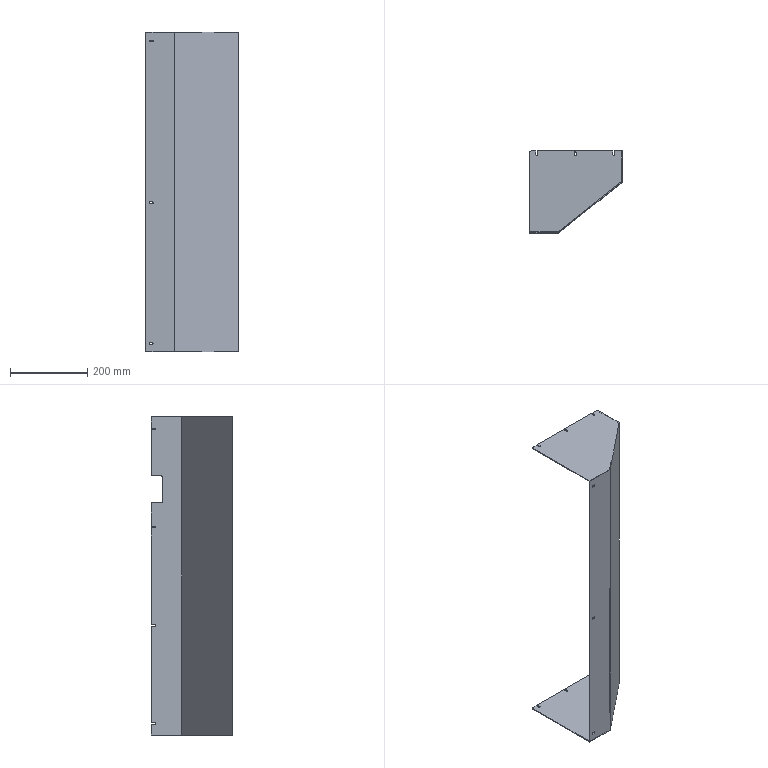Part | NX | features BREP 1 | 1 solid | 72 faces | box 240 x 212 x 830 mm | volume 756946 mm3 | plane 50 | cylinder 22 | commonest cylinder face diameters 4.5 x18 10 x4